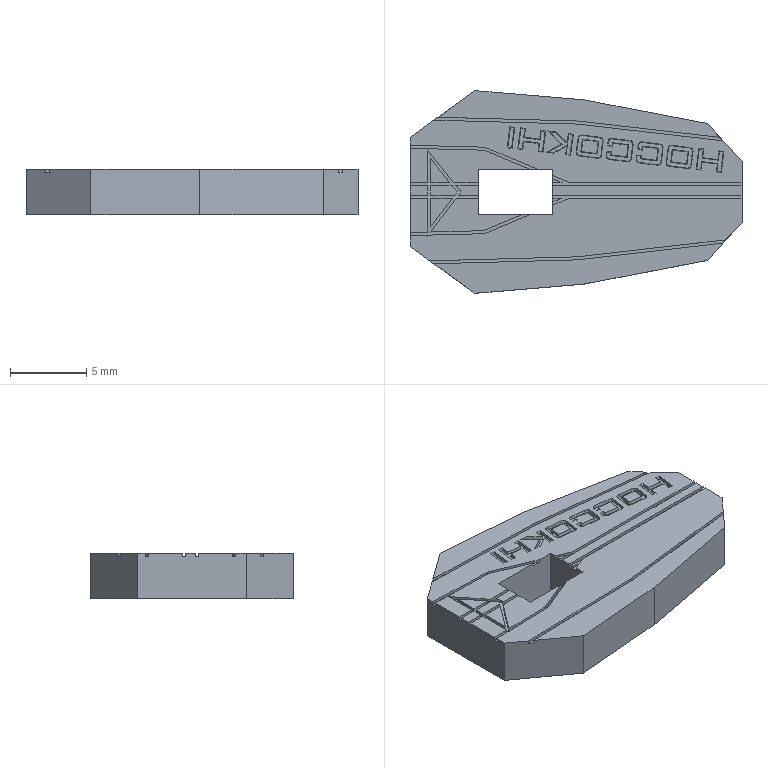Part | SolidWorks | features BaseBody 1 | 1 solid | 197 faces | box 21.822 x 13.322 x 3 mm | volume 656.047 mm3 | plane 173 | spline 24